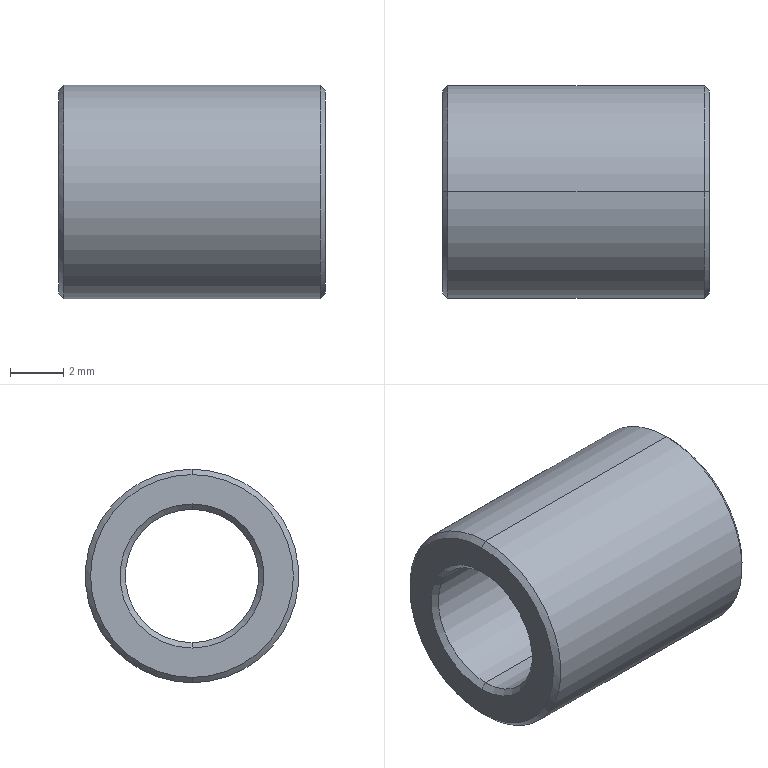Part | STEP file | KNCLM5-8-10 | 1 solid | 14 faces | box 10 x 8 x 8 mm | volume 304.672 mm3 | cone 8 | cylinder 4 | plane 2 | commonest cylinder face diameters 5 x2 8 x2
STEP:
#1=CARTESIAN_POINT('',(0.,0.,0.));
#2=DIRECTION('',(0.,0.,1.));
#3=DIRECTION('',(1.,0.,0.));
#4=AXIS2_PLACEMENT_3D('',#1,#2,#3);
#5=CARTESIAN_POINT('',(24.,0.,-3.8));
#6=VERTEX_POINT('',#5);
#7=CARTESIAN_POINT('',(24.,0.,3.8));
#8=VERTEX_POINT('',#7);
#9=CARTESIAN_POINT('',(24.,0.,0.));
#10=DIRECTION('',(1.,0.,0.));
#11=DIRECTION('',(0.,0.,1.));
#12=AXIS2_PLACEMENT_3D('',#9,#10,#11);
#13=CIRCLE('',#12,3.8);
#14=CARTESIAN_POINT('',(23.8,0.,0.));
#15=DIRECTION('',(-1.,0.,0.));
#16=DIRECTION('',(0.,0.,1.));
#17=AXIS2_PLACEMENT_3D('',#14,#15,#16);
#18=CONICAL_SURFACE('',#17,4.,0.7854);
#19=CARTESIAN_POINT('',(6.283,-0.2));
#20=DIRECTION('',(-1.,0.));
#21=VECTOR('',#20,1.);
#22=LINE('',#19,#21);
#23=(GEOMETRIC_REPRESENTATION_CONTEXT(2)PARAMETRIC_REPRESENTATION_CONTEXT()REPRESENTATION_CONTEXT('',''));
#24=DEFINITIONAL_REPRESENTATION('',(#22),#23);
#25=PCURVE('',#18,#24);
#26=CARTESIAN_POINT('',(24.,2.5,0.));
#27=DIRECTION('',(-1.,0.,0.));
#28=DIRECTION('',(0.,0.,1.));
#29=AXIS2_PLACEMENT_3D('',#26,#27,#28);
#30=PLANE('',#29);
#31=CARTESIAN_POINT('',(3.8,-2.5));
#32=CARTESIAN_POINT('',(3.8,-9.082));
#33=CARTESIAN_POINT('',(-1.9,-5.791));
#34=CARTESIAN_POINT('',(-7.6,-2.5));
#35=CARTESIAN_POINT('',(-1.9,0.7909));
#36=CARTESIAN_POINT('',(3.8,4.082));
#37=CARTESIAN_POINT('',(3.8,-2.5));
#38=(BOUNDED_CURVE()B_SPLINE_CURVE(2,(#31,#32,#33,#34,#35,#36,#37),.UNSPECIFIED.,.T.,.F.)B_SPLINE_CURVE_WITH_KNOTS((1,2,2,2,2,1),(-2.094,0.,2.094,4.189,6.283,8.378),.UNSPECIFIED.)CURVE()GEOMETRIC_REPRESENTATION_ITEM()RATIONAL_B_SPLINE_CURVE((1.,0.5,1.,0.5,1.,0.5,1.))REPRESENTATION_ITEM(''));
#39=(GEOMETRIC_REPRESENTATION_CONTEXT(2)PARAMETRIC_REPRESENTATION_CONTEXT()REPRESENTATION_CONTEXT('',''));
#40=DEFINITIONAL_REPRESENTATION('',(#38),#39);
#41=PCURVE('',#30,#40);
#42=SURFACE_CURVE('',#13,(#25,#41),.PCURVE_S1.);
#43=EDGE_CURVE('',#6,#8,#42,.T.);
#44=ORIENTED_EDGE('',*,*,#43,.F.);
#45=CARTESIAN_POINT('',(23.8,0.,-4.));
#46=VERTEX_POINT('',#45);
#47=CARTESIAN_POINT('',(23.8,0.,-4.));
#48=DIRECTION('',(-0.7071,0.,-0.7071));
#49=VECTOR('',#48,1.);
#50=LINE('',#47,#49);
#51=CARTESIAN_POINT('',(3.142,0.));
#52=DIRECTION('',(0.,1.));
#53=VECTOR('',#52,1.);
#54=LINE('',#51,#53);
#55=(GEOMETRIC_REPRESENTATION_CONTEXT(2)PARAMETRIC_REPRESENTATION_CONTEXT()REPRESENTATION_CONTEXT('',''));
#56=DEFINITIONAL_REPRESENTATION('',(#54),#55);
#57=PCURVE('',#18,#56);
#58=CARTESIAN_POINT('',(23.8,0.,0.));
#59=DIRECTION('',(-1.,0.,0.));
#60=DIRECTION('',(0.,0.,1.));
#61=AXIS2_PLACEMENT_3D('',#58,#59,#60);
#62=CONICAL_SURFACE('',#61,4.,0.7854);
#63=CARTESIAN_POINT('',(3.142,0.));
#64=DIRECTION('',(0.,1.));
#65=VECTOR('',#64,1.);
#66=LINE('',#63,#65);
#67=(GEOMETRIC_REPRESENTATION_CONTEXT(2)PARAMETRIC_REPRESENTATION_CONTEXT()REPRESENTATION_CONTEXT('',''));
#68=DEFINITIONAL_REPRESENTATION('',(#66),#67);
#69=PCURVE('',#62,#68);
#70=SURFACE_CURVE('',#50,(#57,#69),.PCURVE_S1.);
#71=EDGE_CURVE('',#6,#46,#70,.T.);
#72=ORIENTED_EDGE('',*,*,#71,.T.);
#73=CARTESIAN_POINT('',(23.8,0.,4.));
#74=VERTEX_POINT('',#73);
#75=CARTESIAN_POINT('',(23.8,0.,0.));
#76=DIRECTION('',(-1.,0.,0.));
#77=DIRECTION('',(0.,0.,1.));
#78=AXIS2_PLACEMENT_3D('',#75,#76,#77);
#79=CIRCLE('',#78,4.);
#80=CARTESIAN_POINT('',(0.,0.));
#81=DIRECTION('',(1.,0.));
#82=VECTOR('',#81,1.);
#83=LINE('',#80,#82);
#84=(GEOMETRIC_REPRESENTATION_CONTEXT(2)PARAMETRIC_REPRESENTATION_CONTEXT()REPRESENTATION_CONTEXT('',''));
#85=DEFINITIONAL_REPRESENTATION('',(#83),#84);
#86=PCURVE('',#18,#85);
#87=CARTESIAN_POINT('',(14.,0.,0.));
#88=DIRECTION('',(-1.,0.,0.));
#89=DIRECTION('',(0.,0.,1.));
#90=AXIS2_PLACEMENT_3D('',#87,#88,#89);
#91=CYLINDRICAL_SURFACE('',#90,4.);
#92=CARTESIAN_POINT('',(0.,-9.8));
#93=DIRECTION('',(1.,0.));
#94=VECTOR('',#93,1.);
#95=LINE('',#92,#94);
#96=(GEOMETRIC_REPRESENTATION_CONTEXT(2)PARAMETRIC_REPRESENTATION_CONTEXT()REPRESENTATION_CONTEXT('',''));
#97=DEFINITIONAL_REPRESENTATION('',(#95),#96);
#98=PCURVE('',#91,#97);
#99=SURFACE_CURVE('',#79,(#86,#98),.PCURVE_S1.);
#100=EDGE_CURVE('',#74,#46,#99,.T.);
#101=ORIENTED_EDGE('',*,*,#100,.F.);
#102=CARTESIAN_POINT('',(23.8,0.,4.));
#103=DIRECTION('',(-0.7071,0.,0.7071));
#104=VECTOR('',#103,1.);
#105=LINE('',#102,#104);
#106=CARTESIAN_POINT('',(0.,0.));
#107=DIRECTION('',(0.,1.));
#108=VECTOR('',#107,1.);
#109=LINE('',#106,#108);
#110=(GEOMETRIC_REPRESENTATION_CONTEXT(2)PARAMETRIC_REPRESENTATION_CONTEXT()REPRESENTATION_CONTEXT('',''));
#111=DEFINITIONAL_REPRESENTATION('',(#109),#110);
#112=PCURVE('',#18,#111);
#113=CARTESIAN_POINT('',(6.283,0.));
#114=DIRECTION('',(0.,1.));
#115=VECTOR('',#114,1.);
#116=LINE('',#113,#115);
#117=(GEOMETRIC_REPRESENTATION_CONTEXT(2)PARAMETRIC_REPRESENTATION_CONTEXT()REPRESENTATION_CONTEXT('',''));
#118=DEFINITIONAL_REPRESENTATION('',(#116),#117);
#119=PCURVE('',#62,#118);
#120=SURFACE_CURVE('',#105,(#112,#119),.PCURVE_S1.);
#121=EDGE_CURVE('',#8,#74,#120,.T.);
#122=ORIENTED_EDGE('',*,*,#121,.F.);
#123=EDGE_LOOP('',(#44,#72,#101,#122));
#124=FACE_BOUND('',#123,.T.);
#125=ADVANCED_FACE('',(#124),#18,.T.);
#126=CARTESIAN_POINT('',(23.8,0.,-2.5));
#127=VERTEX_POINT('',#126);
#128=CARTESIAN_POINT('',(24.,0.,-2.7));
#129=VERTEX_POINT('',#128);
#130=CARTESIAN_POINT('',(24.,0.,-2.7));
#131=DIRECTION('',(0.7071,0.,-0.7071));
#132=VECTOR('',#131,1.);
#133=LINE('',#130,#132);
#134=CARTESIAN_POINT('',(24.,0.,0.));
#135=DIRECTION('',(1.,0.,0.));
#136=DIRECTION('',(0.,0.,-1.));
#137=AXIS2_PLACEMENT_3D('',#134,#135,#136);
#138=CONICAL_SURFACE('',#137,2.7,0.7854);
#139=CARTESIAN_POINT('',(6.283,0.));
#140=DIRECTION('',(0.,1.));
#141=VECTOR('',#140,1.);
#142=LINE('',#139,#141);
#143=(GEOMETRIC_REPRESENTATION_CONTEXT(2)PARAMETRIC_REPRESENTATION_CONTEXT()REPRESENTATION_CONTEXT('',''));
#144=DEFINITIONAL_REPRESENTATION('',(#142),#143);
#145=PCURVE('',#138,#144);
#146=CARTESIAN_POINT('',(24.,0.,0.));
#147=DIRECTION('',(1.,0.,0.));
#148=DIRECTION('',(0.,0.,-1.));
#149=AXIS2_PLACEMENT_3D('',#146,#147,#148);
#150=CONICAL_SURFACE('',#149,2.7,0.7854);
#151=CARTESIAN_POINT('',(0.,0.));
#152=DIRECTION('',(0.,1.));
#153=VECTOR('',#152,1.);
#154=LINE('',#151,#153);
#155=(GEOMETRIC_REPRESENTATION_CONTEXT(2)PARAMETRIC_REPRESENTATION_CONTEXT()REPRESENTATION_CONTEXT('',''));
#156=DEFINITIONAL_REPRESENTATION('',(#154),#155);
#157=PCURVE('',#150,#156);
#158=SURFACE_CURVE('',#133,(#145,#157),.PCURVE_S1.);
#159=EDGE_CURVE('',#127,#129,#158,.T.);
#160=ORIENTED_EDGE('',*,*,#159,.T.);
#161=CARTESIAN_POINT('',(24.,0.,2.7));
#162=VERTEX_POINT('',#161);
#163=CARTESIAN_POINT('',(24.,0.,0.));
#164=DIRECTION('',(-1.,0.,0.));
#165=DIRECTION('',(0.,0.,1.));
#166=AXIS2_PLACEMENT_3D('',#163,#164,#165);
#167=CIRCLE('',#166,2.7);
#168=CARTESIAN_POINT('',(9.425,0.));
#169=DIRECTION('',(-1.,0.));
#170=VECTOR('',#169,1.);
#171=LINE('',#168,#170);
#172=(GEOMETRIC_REPRESENTATION_CONTEXT(2)PARAMETRIC_REPRESENTATION_CONTEXT()REPRESENTATION_CONTEXT('',''));
#173=DEFINITIONAL_REPRESENTATION('',(#171),#172);
#174=PCURVE('',#138,#173);
#175=CARTESIAN_POINT('',(0.,-2.5));
#176=DIRECTION('',(1.,0.));
#177=AXIS2_PLACEMENT_2D('',#175,#176);
#178=CIRCLE('',#177,2.7);
#179=(GEOMETRIC_REPRESENTATION_CONTEXT(2)PARAMETRIC_REPRESENTATION_CONTEXT()REPRESENTATION_CONTEXT('',''));
#180=DEFINITIONAL_REPRESENTATION('',(#178),#179);
#181=PCURVE('',#30,#180);
#182=SURFACE_CURVE('',#167,(#174,#181),.PCURVE_S1.);
#183=EDGE_CURVE('',#129,#162,#182,.T.);
#184=ORIENTED_EDGE('',*,*,#183,.T.);
#185=CARTESIAN_POINT('',(23.8,0.,2.5));
#186=VERTEX_POINT('',#185);
#187=CARTESIAN_POINT('',(24.,0.,2.7));
#188=DIRECTION('',(0.7071,0.,0.7071));
#189=VECTOR('',#188,1.);
#190=LINE('',#187,#189);
#191=CARTESIAN_POINT('',(3.142,0.));
#192=DIRECTION('',(0.,1.));
#193=VECTOR('',#192,1.);
#194=LINE('',#191,#193);
#195=(GEOMETRIC_REPRESENTATION_CONTEXT(2)PARAMETRIC_REPRESENTATION_CONTEXT()REPRESENTATION_CONTEXT('',''));
#196=DEFINITIONAL_REPRESENTATION('',(#194),#195);
#197=PCURVE('',#138,#196);
#198=CARTESIAN_POINT('',(3.142,0.));
#199=DIRECTION('',(0.,1.));
#200=VECTOR('',#199,1.);
#201=LINE('',#198,#200);
#202=(GEOMETRIC_REPRESENTATION_CONTEXT(2)PARAMETRIC_REPRESENTATION_CONTEXT()REPRESENTATION_CONTEXT('',''));
#203=DEFINITIONAL_REPRESENTATION('',(#201),#202);
#204=PCURVE('',#150,#203);
#205=SURFACE_CURVE('',#190,(#197,#204),.PCURVE_S1.);
#206=EDGE_CURVE('',#186,#162,#205,.T.);
#207=ORIENTED_EDGE('',*,*,#206,.F.);
#208=CARTESIAN_POINT('',(23.8,0.,0.));
#209=DIRECTION('',(1.,0.,0.));
#210=DIRECTION('',(0.,0.,1.));
#211=AXIS2_PLACEMENT_3D('',#208,#209,#210);
#212=CIRCLE('',#211,2.5);
#213=CARTESIAN_POINT('',(3.142,-0.2));
#214=DIRECTION('',(1.,0.));
#215=VECTOR('',#214,1.);
#216=LINE('',#213,#215);
#217=(GEOMETRIC_REPRESENTATION_CONTEXT(2)PARAMETRIC_REPRESENTATION_CONTEXT()REPRESENTATION_CONTEXT('',''));
#218=DEFINITIONAL_REPRESENTATION('',(#216),#217);
#219=PCURVE('',#138,#218);
#220=CARTESIAN_POINT('',(14.,0.,0.));
#221=DIRECTION('',(-1.,0.,0.));
#222=DIRECTION('',(0.,0.,1.));
#223=AXIS2_PLACEMENT_3D('',#220,#221,#222);
#224=CYLINDRICAL_SURFACE('',#223,2.5);
#225=CARTESIAN_POINT('',(6.283,-9.8));
#226=DIRECTION('',(-1.,0.));
#227=VECTOR('',#226,1.);
#228=LINE('',#225,#227);
#229=(GEOMETRIC_REPRESENTATION_CONTEXT(2)PARAMETRIC_REPRESENTATION_CONTEXT()REPRESENTATION_CONTEXT('',''));
#230=DEFINITIONAL_REPRESENTATION('',(#228),#229);
#231=PCURVE('',#224,#230);
#232=SURFACE_CURVE('',#212,(#219,#231),.PCURVE_S1.);
#233=EDGE_CURVE('',#186,#127,#232,.T.);
#234=ORIENTED_EDGE('',*,*,#233,.T.);
#235=EDGE_LOOP('',(#160,#184,#207,#234));
#236=FACE_BOUND('',#235,.F.);
#237=ADVANCED_FACE('',(#236),#138,.F.);
#238=CARTESIAN_POINT('',(14.,0.,3.8));
#239=VERTEX_POINT('',#238);
#240=CARTESIAN_POINT('',(14.,0.,-3.8));
#241=VERTEX_POINT('',#240);
#242=CARTESIAN_POINT('',(14.,0.,0.));
#243=DIRECTION('',(-1.,0.,0.));
#244=DIRECTION('',(0.,0.,-1.));
#245=AXIS2_PLACEMENT_3D('',#242,#243,#244);
#246=CIRCLE('',#245,3.8);
#247=CARTESIAN_POINT('',(14.,0.,0.));
#248=DIRECTION('',(1.,0.,0.));
#249=DIRECTION('',(0.,0.,-1.));
#250=AXIS2_PLACEMENT_3D('',#247,#248,#249);
#251=CONICAL_SURFACE('',#250,3.8,0.7854);
#252=CARTESIAN_POINT('',(6.283,0.));
#253=DIRECTION('',(-1.,0.));
#254=VECTOR('',#253,1.);
#255=LINE('',#252,#254);
#256=(GEOMETRIC_REPRESENTATION_CONTEXT(2)PARAMETRIC_REPRESENTATION_CONTEXT()REPRESENTATION_CONTEXT('',''));
#257=DEFINITIONAL_REPRESENTATION('',(#255),#256);
#258=PCURVE('',#251,#257);
#259=CARTESIAN_POINT('',(14.,2.5,0.));
#260=DIRECTION('',(1.,0.,0.));
#261=DIRECTION('',(0.,0.,-1.));
#262=AXIS2_PLACEMENT_3D('',#259,#260,#261);
#263=PLANE('',#262);
#264=CARTESIAN_POINT('',(3.8,-2.5));
#265=CARTESIAN_POINT('',(3.8,-9.082));
#266=CARTESIAN_POINT('',(-1.9,-5.791));
#267=CARTESIAN_POINT('',(-7.6,-2.5));
#268=CARTESIAN_POINT('',(-1.9,0.7909));
#269=CARTESIAN_POINT('',(3.8,4.082));
#270=CARTESIAN_POINT('',(3.8,-2.5));
#271=(BOUNDED_CURVE()B_SPLINE_CURVE(2,(#264,#265,#266,#267,#268,#269,#270),.UNSPECIFIED.,.T.,.F.)B_SPLINE_CURVE_WITH_KNOTS((1,2,2,2,2,1),(-2.094,0.,2.094,4.189,6.283,8.378),.UNSPECIFIED.)CURVE()GEOMETRIC_REPRESENTATION_ITEM()RATIONAL_B_SPLINE_CURVE((1.,0.5,1.,0.5,1.,0.5,1.))REPRESENTATION_ITEM(''));
#272=(GEOMETRIC_REPRESENTATION_CONTEXT(2)PARAMETRIC_REPRESENTATION_CONTEXT()REPRESENTATION_CONTEXT('',''));
#273=DEFINITIONAL_REPRESENTATION('',(#271),#272);
#274=PCURVE('',#263,#273);
#275=SURFACE_CURVE('',#246,(#258,#274),.PCURVE_S1.);
#276=EDGE_CURVE('',#239,#241,#275,.T.);
#277=ORIENTED_EDGE('',*,*,#276,.F.);
#278=CARTESIAN_POINT('',(14.2,0.,4.));
#279=VERTEX_POINT('',#278);
#280=CARTESIAN_POINT('',(14.,0.,3.8));
#281=DIRECTION('',(0.7071,0.,0.7071));
#282=VECTOR('',#281,1.);
#283=LINE('',#280,#282);
#284=CARTESIAN_POINT('',(3.142,0.));
#285=DIRECTION('',(0.,1.));
#286=VECTOR('',#285,1.);
#287=LINE('',#284,#286);
#288=(GEOMETRIC_REPRESENTATION_CONTEXT(2)PARAMETRIC_REPRESENTATION_CONTEXT()REPRESENTATION_CONTEXT('',''));
#289=DEFINITIONAL_REPRESENTATION('',(#287),#288);
#290=PCURVE('',#251,#289);
#291=CARTESIAN_POINT('',(14.,0.,0.));
#292=DIRECTION('',(1.,0.,0.));
#293=DIRECTION('',(0.,0.,-1.));
#294=AXIS2_PLACEMENT_3D('',#291,#292,#293);
#295=CONICAL_SURFACE('',#294,3.8,0.7854);
#296=CARTESIAN_POINT('',(3.142,0.));
#297=DIRECTION('',(0.,1.));
#298=VECTOR('',#297,1.);
#299=LINE('',#296,#298);
#300=(GEOMETRIC_REPRESENTATION_CONTEXT(2)PARAMETRIC_REPRESENTATION_CONTEXT()REPRESENTATION_CONTEXT('',''));
#301=DEFINITIONAL_REPRESENTATION('',(#299),#300);
#302=PCURVE('',#295,#301);
#303=SURFACE_CURVE('',#283,(#290,#302),.PCURVE_S1.);
#304=EDGE_CURVE('',#239,#279,#303,.T.);
#305=ORIENTED_EDGE('',*,*,#304,.T.);
#306=CARTESIAN_POINT('',(14.2,0.,-4.));
#307=VERTEX_POINT('',#306);
#308=CARTESIAN_POINT('',(14.2,0.,0.));
#309=DIRECTION('',(1.,0.,0.));
#310=DIRECTION('',(0.,0.,-1.));
#311=AXIS2_PLACEMENT_3D('',#308,#309,#310);
#312=CIRCLE('',#311,4.);
#313=CARTESIAN_POINT('',(0.,0.2));
#314=DIRECTION('',(1.,0.));
#315=VECTOR('',#314,1.);
#316=LINE('',#313,#315);
#317=(GEOMETRIC_REPRESENTATION_CONTEXT(2)PARAMETRIC_REPRESENTATION_CONTEXT()REPRESENTATION_CONTEXT('',''));
#318=DEFINITIONAL_REPRESENTATION('',(#316),#317);
#319=PCURVE('',#251,#318);
#320=CARTESIAN_POINT('',(3.142,-0.2));
#321=DIRECTION('',(-1.,0.));
#322=VECTOR('',#321,1.);
#323=LINE('',#320,#322);
#324=(GEOMETRIC_REPRESENTATION_CONTEXT(2)PARAMETRIC_REPRESENTATION_CONTEXT()REPRESENTATION_CONTEXT('',''));
#325=DEFINITIONAL_REPRESENTATION('',(#323),#324);
#326=PCURVE('',#91,#325);
#327=SURFACE_CURVE('',#312,(#319,#326),.PCURVE_S1.);
#328=EDGE_CURVE('',#307,#279,#327,.T.);
#329=ORIENTED_EDGE('',*,*,#328,.F.);
#330=CARTESIAN_POINT('',(14.,0.,-3.8));
#331=DIRECTION('',(0.7071,0.,-0.7071));
#332=VECTOR('',#331,1.);
#333=LINE('',#330,#332);
#334=CARTESIAN_POINT('',(0.,0.));
#335=DIRECTION('',(0.,1.));
#336=VECTOR('',#335,1.);
#337=LINE('',#334,#336);
#338=(GEOMETRIC_REPRESENTATION_CONTEXT(2)PARAMETRIC_REPRESENTATION_CONTEXT()REPRESENTATION_CONTEXT('',''));
#339=DEFINITIONAL_REPRESENTATION('',(#337),#338);
#340=PCURVE('',#251,#339);
#341=CARTESIAN_POINT('',(6.283,0.));
#342=DIRECTION('',(0.,1.));
#343=VECTOR('',#342,1.);
#344=LINE('',#341,#343);
#345=(GEOMETRIC_REPRESENTATION_CONTEXT(2)PARAMETRIC_REPRESENTATION_CONTEXT()REPRESENTATION_CONTEXT('',''));
#346=DEFINITIONAL_REPRESENTATION('',(#344),#345);
#347=PCURVE('',#295,#346);
#348=SURFACE_CURVE('',#333,(#340,#347),.PCURVE_S1.);
#349=EDGE_CURVE('',#241,#307,#348,.T.);
#350=ORIENTED_EDGE('',*,*,#349,.F.);
#351=EDGE_LOOP('',(#277,#305,#329,#350));
#352=FACE_BOUND('',#351,.T.);
#353=ADVANCED_FACE('',(#352),#251,.T.);
#354=CARTESIAN_POINT('',(14.2,0.,2.5));
#355=VERTEX_POINT('',#354);
#356=CARTESIAN_POINT('',(14.,0.,2.7));
#357=VERTEX_POINT('',#356);
#358=CARTESIAN_POINT('',(14.2,0.,2.5));
#359=DIRECTION('',(-0.7071,0.,0.7071));
#360=VECTOR('',#359,1.);
#361=LINE('',#358,#360);
#362=CARTESIAN_POINT('',(14.2,0.,0.));
#363=DIRECTION('',(-1.,0.,0.));
#364=DIRECTION('',(0.,0.,1.));
#365=AXIS2_PLACEMENT_3D('',#362,#363,#364);
#366=CONICAL_SURFACE('',#365,2.5,0.7854);
#367=CARTESIAN_POINT('',(6.283,0.));
#368=DIRECTION('',(0.,1.));
#369=VECTOR('',#368,1.);
#370=LINE('',#367,#369);
#371=(GEOMETRIC_REPRESENTATION_CONTEXT(2)PARAMETRIC_REPRESENTATION_CONTEXT()REPRESENTATION_CONTEXT('',''));
#372=DEFINITIONAL_REPRESENTATION('',(#370),#371);
#373=PCURVE('',#366,#372);
#374=CARTESIAN_POINT('',(14.2,0.,0.));
#375=DIRECTION('',(-1.,0.,0.));
#376=DIRECTION('',(0.,0.,1.));
#377=AXIS2_PLACEMENT_3D('',#374,#375,#376);
#378=CONICAL_SURFACE('',#377,2.5,0.7854);
#379=CARTESIAN_POINT('',(0.,0.));
#380=DIRECTION('',(0.,1.));
#381=VECTOR('',#380,1.);
#382=LINE('',#379,#381);
#383=(GEOMETRIC_REPRESENTATION_CONTEXT(2)PARAMETRIC_REPRESENTATION_CONTEXT()REPRESENTATION_CONTEXT('',''));
#384=DEFINITIONAL_REPRESENTATION('',(#382),#383);
#385=PCURVE('',#378,#384);
#386=SURFACE_CURVE('',#361,(#373,#385),.PCURVE_S1.);
#387=EDGE_CURVE('',#355,#357,#386,.T.);
#388=ORIENTED_EDGE('',*,*,#387,.T.);
#389=CARTESIAN_POINT('',(14.,0.,-2.7));
#390=VERTEX_POINT('',#389);
#391=CARTESIAN_POINT('',(14.,0.,0.));
#392=DIRECTION('',(1.,0.,0.));
#393=DIRECTION('',(0.,0.,-1.));
#394=AXIS2_PLACEMENT_3D('',#391,#392,#393);
#395=CIRCLE('',#394,2.7);
#396=CARTESIAN_POINT('',(9.425,0.2));
#397=DIRECTION('',(-1.,0.));
#398=VECTOR('',#397,1.);
#399=LINE('',#396,#398);
#400=(GEOMETRIC_REPRESENTATION_CONTEXT(2)PARAMETRIC_REPRESENTATION_CONTEXT()REPRESENTATION_CONTEXT('',''));
#401=DEFINITIONAL_REPRESENTATION('',(#399),#400);
#402=PCURVE('',#366,#401);
#403=CARTESIAN_POINT('',(0.,-2.5));
#404=DIRECTION('',(1.,0.));
#405=AXIS2_PLACEMENT_2D('',#403,#404);
#406=CIRCLE('',#405,2.7);
#407=(GEOMETRIC_REPRESENTATION_CONTEXT(2)PARAMETRIC_REPRESENTATION_CONTEXT()REPRESENTATION_CONTEXT('',''));
#408=DEFINITIONAL_REPRESENTATION('',(#406),#407);
#409=PCURVE('',#263,#408);
#410=SURFACE_CURVE('',#395,(#402,#409),.PCURVE_S1.);
#411=EDGE_CURVE('',#357,#390,#410,.T.);
#412=ORIENTED_EDGE('',*,*,#411,.T.);
#413=CARTESIAN_POINT('',(14.2,0.,-2.5));
#414=VERTEX_POINT('',#413);
#415=CARTESIAN_POINT('',(14.2,0.,-2.5));
#416=DIRECTION('',(-0.7071,0.,-0.7071));
#417=VECTOR('',#416,1.);
#418=LINE('',#415,#417);
#419=CARTESIAN_POINT('',(3.142,0.));
#420=DIRECTION('',(0.,1.));
#421=VECTOR('',#420,1.);
#422=LINE('',#419,#421);
#423=(GEOMETRIC_REPRESENTATION_CONTEXT(2)PARAMETRIC_REPRESENTATION_CONTEXT()REPRESENTATION_CONTEXT('',''));
#424=DEFINITIONAL_REPRESENTATION('',(#422),#423);
#425=PCURVE('',#366,#424);
#426=CARTESIAN_POINT('',(3.142,0.));
#427=DIRECTION('',(0.,1.));
#428=VECTOR('',#427,1.);
#429=LINE('',#426,#428);
#430=(GEOMETRIC_REPRESENTATION_CONTEXT(2)PARAMETRIC_REPRESENTATION_CONTEXT()REPRESENTATION_CONTEXT('',''));
#431=DEFINITIONAL_REPRESENTATION('',(#429),#430);
#432=PCURVE('',#378,#431);
#433=SURFACE_CURVE('',#418,(#425,#432),.PCURVE_S1.);
#434=EDGE_CURVE('',#414,#390,#433,.T.);
#435=ORIENTED_EDGE('',*,*,#434,.F.);
#436=CARTESIAN_POINT('',(14.2,0.,0.));
#437=DIRECTION('',(-1.,0.,0.));
#438=DIRECTION('',(0.,0.,-1.));
#439=AXIS2_PLACEMENT_3D('',#436,#437,#438);
#440=CIRCLE('',#439,2.5);
#441=CARTESIAN_POINT('',(3.142,0.));
#442=DIRECTION('',(1.,0.));
#443=VECTOR('',#442,1.);
#444=LINE('',#441,#443);
#445=(GEOMETRIC_REPRESENTATION_CONTEXT(2)PARAMETRIC_REPRESENTATION_CONTEXT()REPRESENTATION_CONTEXT('',''));
#446=DEFINITIONAL_REPRESENTATION('',(#444),#445);
#447=PCURVE('',#366,#446);
#448=CARTESIAN_POINT('',(3.142,-0.2));
#449=DIRECTION('',(1.,0.));
#450=VECTOR('',#449,1.);
#451=LINE('',#448,#450);
#452=(GEOMETRIC_REPRESENTATION_CONTEXT(2)PARAMETRIC_REPRESENTATION_CONTEXT()REPRESENTATION_CONTEXT('',''));
#453=DEFINITIONAL_REPRESENTATION('',(#451),#452);
#454=PCURVE('',#224,#453);
#455=SURFACE_CURVE('',#440,(#447,#454),.PCURVE_S1.);
#456=EDGE_CURVE('',#414,#355,#455,.T.);
#457=ORIENTED_EDGE('',*,*,#456,.T.);
#458=EDGE_LOOP('',(#388,#412,#435,#457));
#459=FACE_BOUND('',#458,.F.);
#460=ADVANCED_FACE('',(#459),#366,.F.);
#461=CARTESIAN_POINT('',(14.,0.,2.5));
#462=DIRECTION('',(-1.,0.,0.));
#463=VECTOR('',#462,1.);
#464=LINE('',#461,#463);
#465=CARTESIAN_POINT('',(6.283,0.));
#466=DIRECTION('',(0.,1.));
#467=VECTOR('',#466,1.);
#468=LINE('',#465,#467);
#469=(GEOMETRIC_REPRESENTATION_CONTEXT(2)PARAMETRIC_REPRESENTATION_CONTEXT()REPRESENTATION_CONTEXT('',''));
#470=DEFINITIONAL_REPRESENTATION('',(#468),#469);
#471=PCURVE('',#224,#470);
#472=CARTESIAN_POINT('',(14.,0.,0.));
#473=DIRECTION('',(-1.,0.,0.));
#474=DIRECTION('',(0.,0.,1.));
#475=AXIS2_PLACEMENT_3D('',#472,#473,#474);
#476=CYLINDRICAL_SURFACE('',#475,2.5);
#477=CARTESIAN_POINT('',(0.,0.));
#478=DIRECTION('',(0.,1.));
#479=VECTOR('',#478,1.);
#480=LINE('',#477,#479);
#481=(GEOMETRIC_REPRESENTATION_CONTEXT(2)PARAMETRIC_REPRESENTATION_CONTEXT()REPRESENTATION_CONTEXT('',''));
#482=DEFINITIONAL_REPRESENTATION('',(#480),#481);
#483=PCURVE('',#476,#482);
#484=SURFACE_CURVE('',#464,(#471,#483),.PCURVE_S1.);
#485=EDGE_CURVE('',#186,#355,#484,.T.);
#486=ORIENTED_EDGE('',*,*,#485,.T.);
#487=ORIENTED_EDGE('',*,*,#456,.F.);
#488=CARTESIAN_POINT('',(14.,0.,-2.5));
#489=DIRECTION('',(-1.,0.,0.));
#490=VECTOR('',#489,1.);
#491=LINE('',#488,#490);
#492=CARTESIAN_POINT('',(3.142,0.));
#493=DIRECTION('',(0.,1.));
#494=VECTOR('',#493,1.);
#495=LINE('',#492,#494);
#496=(GEOMETRIC_REPRESENTATION_CONTEXT(2)PARAMETRIC_REPRESENTATION_CONTEXT()REPRESENTATION_CONTEXT('',''));
#497=DEFINITIONAL_REPRESENTATION('',(#495),#496);
#498=PCURVE('',#224,#497);
#499=CARTESIAN_POINT('',(3.142,0.));
#500=DIRECTION('',(0.,1.));
#501=VECTOR('',#500,1.);
#502=LINE('',#499,#501);
#503=(GEOMETRIC_REPRESENTATION_CONTEXT(2)PARAMETRIC_REPRESENTATION_CONTEXT()REPRESENTATION_CONTEXT('',''));
#504=DEFINITIONAL_REPRESENTATION('',(#502),#503);
#505=PCURVE('',#476,#504);
#506=SURFACE_CURVE('',#491,(#498,#505),.PCURVE_S1.);
#507=EDGE_CURVE('',#127,#414,#506,.T.);
#508=ORIENTED_EDGE('',*,*,#507,.F.);
#509=ORIENTED_EDGE('',*,*,#233,.F.);
#510=EDGE_LOOP('',(#486,#487,#508,#509));
#511=FACE_BOUND('',#510,.F.);
#512=ADVANCED_FACE('',(#511),#224,.F.);
#513=ORIENTED_EDGE('',*,*,#100,.T.);
#514=CARTESIAN_POINT('',(14.,0.,-4.));
#515=DIRECTION('',(-1.,0.,0.));
#516=VECTOR('',#515,1.);
#517=LINE('',#514,#516);
#518=CARTESIAN_POINT('',(3.142,0.));
#519=DIRECTION('',(0.,1.));
#520=VECTOR('',#519,1.);
#521=LINE('',#518,#520);
#522=(GEOMETRIC_REPRESENTATION_CONTEXT(2)PARAMETRIC_REPRESENTATION_CONTEXT()REPRESENTATION_CONTEXT('',''));
#523=DEFINITIONAL_REPRESENTATION('',(#521),#522);
#524=PCURVE('',#91,#523);
#525=CARTESIAN_POINT('',(14.,0.,0.));
#526=DIRECTION('',(-1.,0.,0.));
#527=DIRECTION('',(0.,0.,1.));
#528=AXIS2_PLACEMENT_3D('',#525,#526,#527);
#529=CYLINDRICAL_SURFACE('',#528,4.);
#530=CARTESIAN_POINT('',(3.142,0.));
#531=DIRECTION('',(0.,1.));
#532=VECTOR('',#531,1.);
#533=LINE('',#530,#532);
#534=(GEOMETRIC_REPRESENTATION_CONTEXT(2)PARAMETRIC_REPRESENTATION_CONTEXT()REPRESENTATION_CONTEXT('',''));
#535=DEFINITIONAL_REPRESENTATION('',(#533),#534);
#536=PCURVE('',#529,#535);
#537=SURFACE_CURVE('',#517,(#524,#536),.PCURVE_S1.);
#538=EDGE_CURVE('',#46,#307,#537,.T.);
#539=ORIENTED_EDGE('',*,*,#538,.T.);
#540=ORIENTED_EDGE('',*,*,#328,.T.);
#541=CARTESIAN_POINT('',(14.,0.,4.));
#542=DIRECTION('',(-1.,0.,0.));
#543=VECTOR('',#542,1.);
#544=LINE('',#541,#543);
#545=CARTESIAN_POINT('',(0.,0.));
#546=DIRECTION('',(0.,1.));
#547=VECTOR('',#546,1.);
#548=LINE('',#545,#547);
#549=(GEOMETRIC_REPRESENTATION_CONTEXT(2)PARAMETRIC_REPRESENTATION_CONTEXT()REPRESENTATION_CONTEXT('',''));
#550=DEFINITIONAL_REPRESENTATION('',(#548),#549);
#551=PCURVE('',#91,#550);
#552=CARTESIAN_POINT('',(6.283,0.));
#553=DIRECTION('',(0.,1.));
#554=VECTOR('',#553,1.);
#555=LINE('',#552,#554);
#556=(GEOMETRIC_REPRESENTATION_CONTEXT(2)PARAMETRIC_REPRESENTATION_CONTEXT()REPRESENTATION_CONTEXT('',''));
#557=DEFINITIONAL_REPRESENTATION('',(#555),#556);
#558=PCURVE('',#529,#557);
#559=SURFACE_CURVE('',#544,(#551,#558),.PCURVE_S1.);
#560=EDGE_CURVE('',#74,#279,#559,.T.);
#561=ORIENTED_EDGE('',*,*,#560,.F.);
#562=EDGE_LOOP('',(#513,#539,#540,#561));
#563=FACE_BOUND('',#562,.T.);
#564=ADVANCED_FACE('',(#563),#91,.T.);
#565=ORIENTED_EDGE('',*,*,#411,.T.);
#566=CARTESIAN_POINT('',(14.,0.,0.));
#567=DIRECTION('',(1.,0.,0.));
#568=DIRECTION('',(0.,0.,-1.));
#569=AXIS2_PLACEMENT_3D('',#566,#567,#568);
#570=CIRCLE('',#569,2.7);
#571=CARTESIAN_POINT('',(0.,-2.5));
#572=DIRECTION('',(1.,0.));
#573=AXIS2_PLACEMENT_2D('',#571,#572);
#574=CIRCLE('',#573,2.7);
#575=(GEOMETRIC_REPRESENTATION_CONTEXT(2)PARAMETRIC_REPRESENTATION_CONTEXT()REPRESENTATION_CONTEXT('',''));
#576=DEFINITIONAL_REPRESENTATION('',(#574),#575);
#577=PCURVE('',#263,#576);
#578=CARTESIAN_POINT('',(3.142,0.2));
#579=DIRECTION('',(-1.,0.));
#580=VECTOR('',#579,1.);
#581=LINE('',#578,#580);
#582=(GEOMETRIC_REPRESENTATION_CONTEXT(2)PARAMETRIC_REPRESENTATION_CONTEXT()REPRESENTATION_CONTEXT('',''));
#583=DEFINITIONAL_REPRESENTATION('',(#581),#582);
#584=PCURVE('',#378,#583);
#585=SURFACE_CURVE('',#570,(#577,#584),.PCURVE_S1.);
#586=EDGE_CURVE('',#390,#357,#585,.T.);
#587=ORIENTED_EDGE('',*,*,#586,.T.);
#588=EDGE_LOOP('',(#565,#587));
#589=FACE_BOUND('',#588,.T.);
#590=CARTESIAN_POINT('',(14.,0.,0.));
#591=DIRECTION('',(-1.,0.,0.));
#592=DIRECTION('',(0.,0.,-1.));
#593=AXIS2_PLACEMENT_3D('',#590,#591,#592);
#594=CIRCLE('',#593,3.8);
#595=CARTESIAN_POINT('',(3.8,-2.5));
#596=CARTESIAN_POINT('',(3.8,-9.082));
#597=CARTESIAN_POINT('',(-1.9,-5.791));
#598=CARTESIAN_POINT('',(-7.6,-2.5));
#599=CARTESIAN_POINT('',(-1.9,0.7909));
#600=CARTESIAN_POINT('',(3.8,4.082));
#601=CARTESIAN_POINT('',(3.8,-2.5));
#602=(BOUNDED_CURVE()B_SPLINE_CURVE(2,(#595,#596,#597,#598,#599,#600,#601),.UNSPECIFIED.,.T.,.F.)B_SPLINE_CURVE_WITH_KNOTS((1,2,2,2,2,1),(-2.094,0.,2.094,4.189,6.283,8.378),.UNSPECIFIED.)CURVE()GEOMETRIC_REPRESENTATION_ITEM()RATIONAL_B_SPLINE_CURVE((1.,0.5,1.,0.5,1.,0.5,1.))REPRESENTATION_ITEM(''));
#603=(GEOMETRIC_REPRESENTATION_CONTEXT(2)PARAMETRIC_REPRESENTATION_CONTEXT()REPRESENTATION_CONTEXT('',''));
#604=DEFINITIONAL_REPRESENTATION('',(#602),#603);
#605=PCURVE('',#263,#604);
#606=CARTESIAN_POINT('',(6.283,0.));
#607=DIRECTION('',(-1.,0.));
#608=VECTOR('',#607,1.);
#609=LINE('',#606,#608);
#610=(GEOMETRIC_REPRESENTATION_CONTEXT(2)PARAMETRIC_REPRESENTATION_CONTEXT()REPRESENTATION_CONTEXT('',''));
#611=DEFINITIONAL_REPRESENTATION('',(#609),#610);
#612=PCURVE('',#295,#611);
#613=SURFACE_CURVE('',#594,(#605,#612),.PCURVE_S1.);
#614=EDGE_CURVE('',#241,#239,#613,.T.);
#615=ORIENTED_EDGE('',*,*,#614,.T.);
#616=ORIENTED_EDGE('',*,*,#276,.T.);
#617=EDGE_LOOP('',(#615,#616));
#618=FACE_BOUND('',#617,.T.);
#619=ADVANCED_FACE('',(#589,#618),#263,.F.);
#620=ORIENTED_EDGE('',*,*,#538,.F.);
#621=CARTESIAN_POINT('',(23.8,0.,0.));
#622=DIRECTION('',(-1.,0.,0.));
#623=DIRECTION('',(0.,0.,1.));
#624=AXIS2_PLACEMENT_3D('',#621,#622,#623);
#625=CIRCLE('',#624,4.);
#626=CARTESIAN_POINT('',(0.,-9.8));
#627=DIRECTION('',(1.,0.));
#628=VECTOR('',#627,1.);
#629=LINE('',#626,#628);
#630=(GEOMETRIC_REPRESENTATION_CONTEXT(2)PARAMETRIC_REPRESENTATION_CONTEXT()REPRESENTATION_CONTEXT('',''));
#631=DEFINITIONAL_REPRESENTATION('',(#629),#630);
#632=PCURVE('',#529,#631);
#633=CARTESIAN_POINT('',(0.,0.));
#634=DIRECTION('',(1.,0.));
#635=VECTOR('',#634,1.);
#636=LINE('',#633,#635);
#637=(GEOMETRIC_REPRESENTATION_CONTEXT(2)PARAMETRIC_REPRESENTATION_CONTEXT()REPRESENTATION_CONTEXT('',''));
#638=DEFINITIONAL_REPRESENTATION('',(#636),#637);
#639=PCURVE('',#62,#638);
#640=SURFACE_CURVE('',#625,(#632,#639),.PCURVE_S1.);
#641=EDGE_CURVE('',#46,#74,#640,.T.);
#642=ORIENTED_EDGE('',*,*,#641,.T.);
#643=ORIENTED_EDGE('',*,*,#560,.T.);
#644=CARTESIAN_POINT('',(14.2,0.,0.));
#645=DIRECTION('',(1.,0.,0.));
#646=DIRECTION('',(0.,0.,-1.));
#647=AXIS2_PLACEMENT_3D('',#644,#645,#646);
#648=CIRCLE('',#647,4.);
#649=CARTESIAN_POINT('',(9.425,-0.2));
#650=DIRECTION('',(-1.,0.));
#651=VECTOR('',#650,1.);
#652=LINE('',#649,#651);
#653=(GEOMETRIC_REPRESENTATION_CONTEXT(2)PARAMETRIC_REPRESENTATION_CONTEXT()REPRESENTATION_CONTEXT('',''));
#654=DEFINITIONAL_REPRESENTATION('',(#652),#653);
#655=PCURVE('',#529,#654);
#656=CARTESIAN_POINT('',(0.,0.2));
#657=DIRECTION('',(1.,0.));
#658=VECTOR('',#657,1.);
#659=LINE('',#656,#658);
#660=(GEOMETRIC_REPRESENTATION_CONTEXT(2)PARAMETRIC_REPRESENTATION_CONTEXT()REPRESENTATION_CONTEXT('',''));
#661=DEFINITIONAL_REPRESENTATION('',(#659),#660);
#662=PCURVE('',#295,#661);
#663=SURFACE_CURVE('',#648,(#655,#662),.PCURVE_S1.);
#664=EDGE_CURVE('',#279,#307,#663,.T.);
#665=ORIENTED_EDGE('',*,*,#664,.T.);
#666=EDGE_LOOP('',(#620,#642,#643,#665));
#667=FACE_BOUND('',#666,.T.);
#668=ADVANCED_FACE('',(#667),#529,.T.);
#669=ORIENTED_EDGE('',*,*,#183,.T.);
#670=CARTESIAN_POINT('',(24.,0.,0.));
#671=DIRECTION('',(-1.,0.,0.));
#672=DIRECTION('',(0.,0.,1.));
#673=AXIS2_PLACEMENT_3D('',#670,#671,#672);
#674=CIRCLE('',#673,2.7);
#675=CARTESIAN_POINT('',(0.,-2.5));
#676=DIRECTION('',(1.,0.));
#677=AXIS2_PLACEMENT_2D('',#675,#676);
#678=CIRCLE('',#677,2.7);
#679=(GEOMETRIC_REPRESENTATION_CONTEXT(2)PARAMETRIC_REPRESENTATION_CONTEXT()REPRESENTATION_CONTEXT('',''));
#680=DEFINITIONAL_REPRESENTATION('',(#678),#679);
#681=PCURVE('',#30,#680);
#682=CARTESIAN_POINT('',(3.142,0.));
#683=DIRECTION('',(-1.,0.));
#684=VECTOR('',#683,1.);
#685=LINE('',#682,#684);
#686=(GEOMETRIC_REPRESENTATION_CONTEXT(2)PARAMETRIC_REPRESENTATION_CONTEXT()REPRESENTATION_CONTEXT('',''));
#687=DEFINITIONAL_REPRESENTATION('',(#685),#686);
#688=PCURVE('',#150,#687);
#689=SURFACE_CURVE('',#674,(#681,#688),.PCURVE_S1.);
#690=EDGE_CURVE('',#162,#129,#689,.T.);
#691=ORIENTED_EDGE('',*,*,#690,.T.);
#692=EDGE_LOOP('',(#669,#691));
#693=FACE_BOUND('',#692,.T.);
#694=CARTESIAN_POINT('',(24.,0.,0.));
#695=DIRECTION('',(1.,0.,0.));
#696=DIRECTION('',(0.,0.,1.));
#697=AXIS2_PLACEMENT_3D('',#694,#695,#696);
#698=CIRCLE('',#697,3.8);
#699=CARTESIAN_POINT('',(3.8,-2.5));
#700=CARTESIAN_POINT('',(3.8,-9.082));
#701=CARTESIAN_POINT('',(-1.9,-5.791));
#702=CARTESIAN_POINT('',(-7.6,-2.5));
#703=CARTESIAN_POINT('',(-1.9,0.7909));
#704=CARTESIAN_POINT('',(3.8,4.082));
#705=CARTESIAN_POINT('',(3.8,-2.5));
#706=(BOUNDED_CURVE()B_SPLINE_CURVE(2,(#699,#700,#701,#702,#703,#704,#705),.UNSPECIFIED.,.T.,.F.)B_SPLINE_CURVE_WITH_KNOTS((1,2,2,2,2,1),(-2.094,0.,2.094,4.189,6.283,8.378),.UNSPECIFIED.)CURVE()GEOMETRIC_REPRESENTATION_ITEM()RATIONAL_B_SPLINE_CURVE((1.,0.5,1.,0.5,1.,0.5,1.))REPRESENTATION_ITEM(''));
#707=(GEOMETRIC_REPRESENTATION_CONTEXT(2)PARAMETRIC_REPRESENTATION_CONTEXT()REPRESENTATION_CONTEXT('',''));
#708=DEFINITIONAL_REPRESENTATION('',(#706),#707);
#709=PCURVE('',#30,#708);
#710=CARTESIAN_POINT('',(6.283,-0.2));
#711=DIRECTION('',(-1.,0.));
#712=VECTOR('',#711,1.);
#713=LINE('',#710,#712);
#714=(GEOMETRIC_REPRESENTATION_CONTEXT(2)PARAMETRIC_REPRESENTATION_CONTEXT()REPRESENTATION_CONTEXT('',''));
#715=DEFINITIONAL_REPRESENTATION('',(#713),#714);
#716=PCURVE('',#62,#715);
#717=SURFACE_CURVE('',#698,(#709,#716),.PCURVE_S1.);
#718=EDGE_CURVE('',#8,#6,#717,.T.);
#719=ORIENTED_EDGE('',*,*,#718,.T.);
#720=ORIENTED_EDGE('',*,*,#43,.T.);
#721=EDGE_LOOP('',(#719,#720));
#722=FACE_BOUND('',#721,.T.);
#723=ADVANCED_FACE('',(#693,#722),#30,.F.);
#724=CARTESIAN_POINT('',(14.2,0.,0.));
#725=DIRECTION('',(-1.,0.,0.));
#726=DIRECTION('',(0.,0.,-1.));
#727=AXIS2_PLACEMENT_3D('',#724,#725,#726);
#728=CIRCLE('',#727,2.5);
#729=CARTESIAN_POINT('',(-3.142,-0.2));
#730=DIRECTION('',(1.,0.));
#731=VECTOR('',#730,1.);
#732=LINE('',#729,#731);
#733=(GEOMETRIC_REPRESENTATION_CONTEXT(2)PARAMETRIC_REPRESENTATION_CONTEXT()REPRESENTATION_CONTEXT('',''));
#734=DEFINITIONAL_REPRESENTATION('',(#732),#733);
#735=PCURVE('',#476,#734);
#736=CARTESIAN_POINT('',(-3.142,0.));
#737=DIRECTION('',(1.,0.));
#738=VECTOR('',#737,1.);
#739=LINE('',#736,#738);
#740=(GEOMETRIC_REPRESENTATION_CONTEXT(2)PARAMETRIC_REPRESENTATION_CONTEXT()REPRESENTATION_CONTEXT('',''));
#741=DEFINITIONAL_REPRESENTATION('',(#739),#740);
#742=PCURVE('',#378,#741);
#743=SURFACE_CURVE('',#728,(#735,#742),.PCURVE_S1.);
#744=EDGE_CURVE('',#355,#414,#743,.T.);
#745=ORIENTED_EDGE('',*,*,#744,.F.);
#746=ORIENTED_EDGE('',*,*,#485,.F.);
#747=CARTESIAN_POINT('',(23.8,0.,0.));
#748=DIRECTION('',(1.,0.,0.));
#749=DIRECTION('',(0.,0.,1.));
#750=AXIS2_PLACEMENT_3D('',#747,#748,#749);
#751=CIRCLE('',#750,2.5);
#752=CARTESIAN_POINT('',(6.283,-9.8));
#753=DIRECTION('',(-1.,0.));
#754=VECTOR('',#753,1.);
#755=LINE('',#752,#754);
#756=(GEOMETRIC_REPRESENTATION_CONTEXT(2)PARAMETRIC_REPRESENTATION_CONTEXT()REPRESENTATION_CONTEXT('',''));
#757=DEFINITIONAL_REPRESENTATION('',(#755),#756);
#758=PCURVE('',#476,#757);
#759=CARTESIAN_POINT('',(-3.142,-0.2));
#760=DIRECTION('',(1.,0.));
#761=VECTOR('',#760,1.);
#762=LINE('',#759,#761);
#763=(GEOMETRIC_REPRESENTATION_CONTEXT(2)PARAMETRIC_REPRESENTATION_CONTEXT()REPRESENTATION_CONTEXT('',''));
#764=DEFINITIONAL_REPRESENTATION('',(#762),#763);
#765=PCURVE('',#150,#764);
#766=SURFACE_CURVE('',#751,(#758,#765),.PCURVE_S1.);
#767=EDGE_CURVE('',#127,#186,#766,.T.);
#768=ORIENTED_EDGE('',*,*,#767,.F.);
#769=ORIENTED_EDGE('',*,*,#507,.T.);
#770=EDGE_LOOP('',(#745,#746,#768,#769));
#771=FACE_BOUND('',#770,.F.);
#772=ADVANCED_FACE('',(#771),#476,.F.);
#773=ORIENTED_EDGE('',*,*,#586,.T.);
#774=ORIENTED_EDGE('',*,*,#387,.F.);
#775=ORIENTED_EDGE('',*,*,#744,.T.);
#776=ORIENTED_EDGE('',*,*,#434,.T.);
#777=EDGE_LOOP('',(#773,#774,#775,#776));
#778=FACE_BOUND('',#777,.F.);
#779=ADVANCED_FACE('',(#778),#378,.F.);
#780=ORIENTED_EDGE('',*,*,#304,.F.);
#781=ORIENTED_EDGE('',*,*,#614,.F.);
#782=ORIENTED_EDGE('',*,*,#349,.T.);
#783=ORIENTED_EDGE('',*,*,#664,.F.);
#784=EDGE_LOOP('',(#780,#781,#782,#783));
#785=FACE_BOUND('',#784,.T.);
#786=ADVANCED_FACE('',(#785),#295,.T.);
#787=ORIENTED_EDGE('',*,*,#690,.T.);
#788=ORIENTED_EDGE('',*,*,#159,.F.);
#789=ORIENTED_EDGE('',*,*,#767,.T.);
#790=ORIENTED_EDGE('',*,*,#206,.T.);
#791=EDGE_LOOP('',(#787,#788,#789,#790));
#792=FACE_BOUND('',#791,.F.);
#793=ADVANCED_FACE('',(#792),#150,.F.);
#794=ORIENTED_EDGE('',*,*,#71,.F.);
#795=ORIENTED_EDGE('',*,*,#718,.F.);
#796=ORIENTED_EDGE('',*,*,#121,.T.);
#797=ORIENTED_EDGE('',*,*,#641,.F.);
#798=EDGE_LOOP('',(#794,#795,#796,#797));
#799=FACE_BOUND('',#798,.T.);
#800=ADVANCED_FACE('',(#799),#62,.T.);
#801=CLOSED_SHELL('',(#125,#237,#353,#460,#512,#564,#619,#668,#723,#772,#779,#786,#793,#800));
#802=MANIFOLD_SOLID_BREP('',#801);
#803=(LENGTH_UNIT()NAMED_UNIT(*)SI_UNIT(.MILLI.,.METRE.));
#804=UNCERTAINTY_MEASURE_WITH_UNIT(LENGTH_MEASURE(0.0000001),#803,'','');
#805=(NAMED_UNIT(*)PLANE_ANGLE_UNIT()SI_UNIT($,.RADIAN.));
#806=(NAMED_UNIT(*)SI_UNIT($,.STERADIAN.)SOLID_ANGLE_UNIT());
#807=(GEOMETRIC_REPRESENTATION_CONTEXT(3)GLOBAL_UNCERTAINTY_ASSIGNED_CONTEXT((#804))GLOBAL_UNIT_ASSIGNED_CONTEXT((#803,#805,#806))REPRESENTATION_CONTEXT('',''));
#808=ADVANCED_BREP_SHAPE_REPRESENTATION('',(#4,#802),#807);